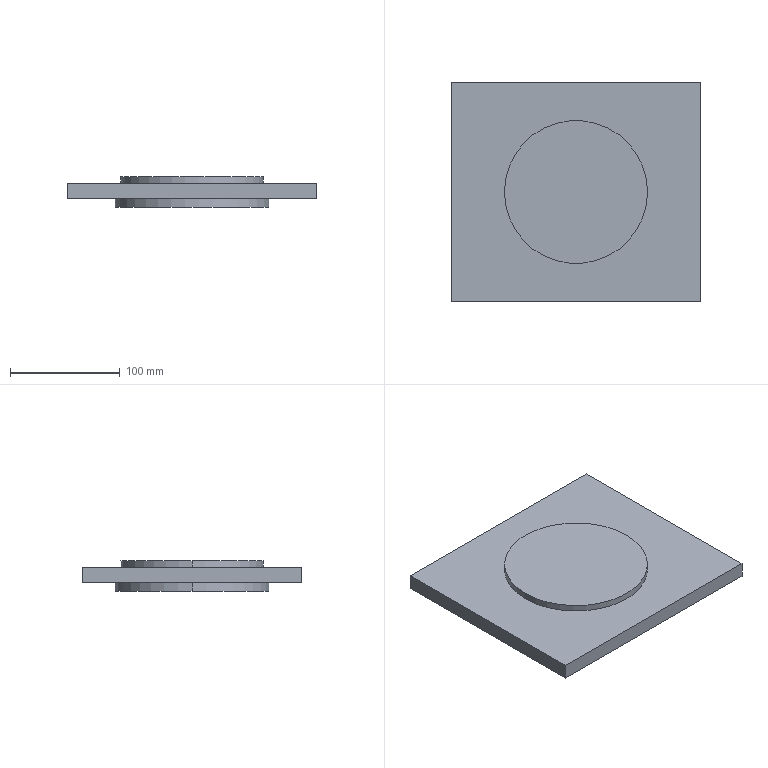Part | SolidWorks | features ICE 2, Extrusion 1 | 1 solid | 12 faces | box 227 x 200 x 28 mm | volume 838390 mm3 | plane 8 | cylinder 4 | commonest cylinder face diameters 130 x2 140 x2
STEP:
#1=CARTESIAN_POINT('',(43.5,100.,-8.));
#2=VERTEX_POINT('',#1);
#3=CARTESIAN_POINT('',(183.5,100.,-8.));
#4=VERTEX_POINT('',#3);
#5=CARTESIAN_POINT('',(113.5,100.,-8.));
#6=DIRECTION('',(0.,0.,-1.));
#7=DIRECTION('',(-1.,0.,0.));
#8=AXIS2_PLACEMENT_3D('',#5,#6,#7);
#9=CIRCLE('',#8,70.);
#10=EDGE_CURVE('',#2,#4,#9,.T.);
#11=ORIENTED_EDGE('',*,*,#10,.F.);
#12=CARTESIAN_POINT('',(43.5,100.,0.));
#13=VERTEX_POINT('',#12);
#14=CARTESIAN_POINT('',(43.5,100.,-8.));
#15=DIRECTION('',(0.,0.,1.));
#16=VECTOR('',#15,1000.);
#17=LINE('',#14,#16);
#18=EDGE_CURVE('',#2,#13,#17,.T.);
#19=ORIENTED_EDGE('',*,*,#18,.T.);
#20=CARTESIAN_POINT('',(183.5,100.,0.));
#21=VERTEX_POINT('',#20);
#22=CARTESIAN_POINT('',(113.5,100.,0.));
#23=DIRECTION('',(0.,0.,-1.));
#24=DIRECTION('',(-1.,0.,0.));
#25=AXIS2_PLACEMENT_3D('',#22,#23,#24);
#26=CIRCLE('',#25,70.);
#27=EDGE_CURVE('',#13,#21,#26,.T.);
#28=ORIENTED_EDGE('',*,*,#27,.T.);
#29=CARTESIAN_POINT('',(183.5,100.,-8.));
#30=DIRECTION('',(0.,0.,1.));
#31=VECTOR('',#30,1000.);
#32=LINE('',#29,#31);
#33=EDGE_CURVE('',#4,#21,#32,.T.);
#34=ORIENTED_EDGE('',*,*,#33,.F.);
#35=EDGE_LOOP('',(#11,#19,#28,#34));
#36=FACE_OUTER_BOUND('',#35,.T.);
#37=CARTESIAN_POINT('',(113.5,100.,-8.));
#38=DIRECTION('',(0.,0.,1.));
#39=DIRECTION('',(1.,0.,0.));
#40=AXIS2_PLACEMENT_3D('',#37,#38,#39);
#41=CYLINDRICAL_SURFACE('',#40,70.);
#42=ADVANCED_FACE('',(#36),#41,.T.);
#43=CARTESIAN_POINT('',(178.5,100.,20.));
#44=VERTEX_POINT('',#43);
#45=CARTESIAN_POINT('',(48.5,100.,20.));
#46=VERTEX_POINT('',#45);
#47=CARTESIAN_POINT('',(113.5,100.,20.));
#48=DIRECTION('',(0.,0.,1.));
#49=DIRECTION('',(1.,0.,0.));
#50=AXIS2_PLACEMENT_3D('',#47,#48,#49);
#51=CIRCLE('',#50,65.);
#52=EDGE_CURVE('',#44,#46,#51,.T.);
#53=ORIENTED_EDGE('',*,*,#52,.F.);
#54=CARTESIAN_POINT('',(178.5,100.,14.));
#55=VERTEX_POINT('',#54);
#56=CARTESIAN_POINT('',(178.5,100.,20.));
#57=DIRECTION('',(0.,0.,-1.));
#58=VECTOR('',#57,1000.);
#59=LINE('',#56,#58);
#60=EDGE_CURVE('',#44,#55,#59,.T.);
#61=ORIENTED_EDGE('',*,*,#60,.T.);
#62=CARTESIAN_POINT('',(48.5,100.,14.));
#63=VERTEX_POINT('',#62);
#64=CARTESIAN_POINT('',(113.5,100.,14.));
#65=DIRECTION('',(0.,0.,1.));
#66=DIRECTION('',(-1.,0.,0.));
#67=AXIS2_PLACEMENT_3D('',#64,#65,#66);
#68=CIRCLE('',#67,65.);
#69=EDGE_CURVE('',#55,#63,#68,.T.);
#70=ORIENTED_EDGE('',*,*,#69,.T.);
#71=CARTESIAN_POINT('',(48.5,100.,20.));
#72=DIRECTION('',(0.,0.,-1.));
#73=VECTOR('',#72,1000.);
#74=LINE('',#71,#73);
#75=EDGE_CURVE('',#46,#63,#74,.T.);
#76=ORIENTED_EDGE('',*,*,#75,.F.);
#77=EDGE_LOOP('',(#53,#61,#70,#76));
#78=FACE_OUTER_BOUND('',#77,.T.);
#79=CARTESIAN_POINT('',(113.5,100.,20.));
#80=DIRECTION('',(0.,0.,-1.));
#81=DIRECTION('',(-1.,0.,0.));
#82=AXIS2_PLACEMENT_3D('',#79,#80,#81);
#83=CYLINDRICAL_SURFACE('',#82,65.);
#84=ADVANCED_FACE('',(#78),#83,.T.);
#85=CARTESIAN_POINT('',(0.,0.,0.));
#86=VERTEX_POINT('',#85);
#87=CARTESIAN_POINT('',(227.,0.,0.));
#88=VERTEX_POINT('',#87);
#89=CARTESIAN_POINT('',(227.,0.,0.));
#90=DIRECTION('',(1.,0.,0.));
#91=VECTOR('',#90,1000.);
#92=LINE('',#89,#91);
#93=EDGE_CURVE('',#86,#88,#92,.T.);
#94=ORIENTED_EDGE('',*,*,#93,.F.);
#95=CARTESIAN_POINT('',(0.,200.,0.));
#96=VERTEX_POINT('',#95);
#97=CARTESIAN_POINT('',(0.,0.,0.));
#98=DIRECTION('',(0.,-1.,0.));
#99=VECTOR('',#98,1000.);
#100=LINE('',#97,#99);
#101=EDGE_CURVE('',#96,#86,#100,.T.);
#102=ORIENTED_EDGE('',*,*,#101,.F.);
#103=CARTESIAN_POINT('',(227.,200.,0.));
#104=VERTEX_POINT('',#103);
#105=CARTESIAN_POINT('',(0.,200.,0.));
#106=DIRECTION('',(-1.,0.,0.));
#107=VECTOR('',#106,1000.);
#108=LINE('',#105,#107);
#109=EDGE_CURVE('',#104,#96,#108,.T.);
#110=ORIENTED_EDGE('',*,*,#109,.F.);
#111=CARTESIAN_POINT('',(227.,200.,0.));
#112=DIRECTION('',(0.,1.,0.));
#113=VECTOR('',#112,1000.);
#114=LINE('',#111,#113);
#115=EDGE_CURVE('',#88,#104,#114,.T.);
#116=ORIENTED_EDGE('',*,*,#115,.F.);
#117=EDGE_LOOP('',(#94,#102,#110,#116));
#118=FACE_OUTER_BOUND('',#117,.T.);
#119=CARTESIAN_POINT('',(113.5,100.,0.));
#120=DIRECTION('',(0.,0.,-1.));
#121=DIRECTION('',(-1.,0.,0.));
#122=AXIS2_PLACEMENT_3D('',#119,#120,#121);
#123=CIRCLE('',#122,70.);
#124=EDGE_CURVE('',#21,#13,#123,.T.);
#125=ORIENTED_EDGE('',*,*,#124,.F.);
#126=ORIENTED_EDGE('',*,*,#27,.F.);
#127=EDGE_LOOP('',(#125,#126));
#128=FACE_BOUND('',#127,.T.);
#129=CARTESIAN_POINT('',(0.,0.,0.));
#130=DIRECTION('',(0.,0.,-1.));
#131=DIRECTION('',(-1.,0.,0.));
#132=AXIS2_PLACEMENT_3D('',#129,#130,#131);
#133=PLANE('',#132);
#134=ADVANCED_FACE('',(#118,#128),#133,.T.);
#135=CARTESIAN_POINT('',(0.,0.,14.));
#136=VERTEX_POINT('',#135);
#137=CARTESIAN_POINT('',(227.,0.,14.));
#138=VERTEX_POINT('',#137);
#139=CARTESIAN_POINT('',(227.,0.,14.));
#140=DIRECTION('',(1.,0.,0.));
#141=VECTOR('',#140,1000.);
#142=LINE('',#139,#141);
#143=EDGE_CURVE('',#136,#138,#142,.T.);
#144=ORIENTED_EDGE('',*,*,#143,.T.);
#145=CARTESIAN_POINT('',(227.,200.,14.));
#146=VERTEX_POINT('',#145);
#147=CARTESIAN_POINT('',(227.,200.,14.));
#148=DIRECTION('',(0.,1.,0.));
#149=VECTOR('',#148,1000.);
#150=LINE('',#147,#149);
#151=EDGE_CURVE('',#138,#146,#150,.T.);
#152=ORIENTED_EDGE('',*,*,#151,.T.);
#153=CARTESIAN_POINT('',(0.,200.,14.));
#154=VERTEX_POINT('',#153);
#155=CARTESIAN_POINT('',(0.,200.,14.));
#156=DIRECTION('',(-1.,0.,0.));
#157=VECTOR('',#156,1000.);
#158=LINE('',#155,#157);
#159=EDGE_CURVE('',#146,#154,#158,.T.);
#160=ORIENTED_EDGE('',*,*,#159,.T.);
#161=CARTESIAN_POINT('',(0.,0.,14.));
#162=DIRECTION('',(0.,-1.,0.));
#163=VECTOR('',#162,1000.);
#164=LINE('',#161,#163);
#165=EDGE_CURVE('',#154,#136,#164,.T.);
#166=ORIENTED_EDGE('',*,*,#165,.T.);
#167=EDGE_LOOP('',(#144,#152,#160,#166));
#168=FACE_OUTER_BOUND('',#167,.T.);
#169=CARTESIAN_POINT('',(113.5,100.,14.));
#170=DIRECTION('',(0.,0.,1.));
#171=DIRECTION('',(-1.,0.,0.));
#172=AXIS2_PLACEMENT_3D('',#169,#170,#171);
#173=CIRCLE('',#172,65.);
#174=EDGE_CURVE('',#63,#55,#173,.T.);
#175=ORIENTED_EDGE('',*,*,#174,.F.);
#176=ORIENTED_EDGE('',*,*,#69,.F.);
#177=EDGE_LOOP('',(#175,#176));
#178=FACE_BOUND('',#177,.T.);
#179=CARTESIAN_POINT('',(0.,0.,14.));
#180=DIRECTION('',(0.,0.,-1.));
#181=DIRECTION('',(-1.,0.,0.));
#182=AXIS2_PLACEMENT_3D('',#179,#180,#181);
#183=PLANE('',#182);
#184=ADVANCED_FACE('',(#168,#178),#183,.F.);
#185=ORIENTED_EDGE('',*,*,#93,.T.);
#186=CARTESIAN_POINT('',(227.,0.,14.));
#187=DIRECTION('',(0.,0.,-1.));
#188=VECTOR('',#187,1000.);
#189=LINE('',#186,#188);
#190=EDGE_CURVE('',#138,#88,#189,.T.);
#191=ORIENTED_EDGE('',*,*,#190,.F.);
#192=ORIENTED_EDGE('',*,*,#143,.F.);
#193=CARTESIAN_POINT('',(0.,0.,14.));
#194=DIRECTION('',(0.,0.,-1.));
#195=VECTOR('',#194,1000.);
#196=LINE('',#193,#195);
#197=EDGE_CURVE('',#136,#86,#196,.T.);
#198=ORIENTED_EDGE('',*,*,#197,.T.);
#199=EDGE_LOOP('',(#185,#191,#192,#198));
#200=FACE_OUTER_BOUND('',#199,.T.);
#201=CARTESIAN_POINT('',(227.,0.,14.));
#202=DIRECTION('',(0.,1.,0.));
#203=DIRECTION('',(-1.,0.,0.));
#204=AXIS2_PLACEMENT_3D('',#201,#202,#203);
#205=PLANE('',#204);
#206=ADVANCED_FACE('',(#200),#205,.F.);
#207=ORIENTED_EDGE('',*,*,#115,.T.);
#208=CARTESIAN_POINT('',(227.,200.,14.));
#209=DIRECTION('',(0.,0.,-1.));
#210=VECTOR('',#209,1000.);
#211=LINE('',#208,#210);
#212=EDGE_CURVE('',#146,#104,#211,.T.);
#213=ORIENTED_EDGE('',*,*,#212,.F.);
#214=ORIENTED_EDGE('',*,*,#151,.F.);
#215=ORIENTED_EDGE('',*,*,#190,.T.);
#216=EDGE_LOOP('',(#207,#213,#214,#215));
#217=FACE_OUTER_BOUND('',#216,.T.);
#218=CARTESIAN_POINT('',(227.,200.,14.));
#219=DIRECTION('',(-1.,0.,0.));
#220=DIRECTION('',(0.,-1.,0.));
#221=AXIS2_PLACEMENT_3D('',#218,#219,#220);
#222=PLANE('',#221);
#223=ADVANCED_FACE('',(#217),#222,.F.);
#224=ORIENTED_EDGE('',*,*,#109,.T.);
#225=CARTESIAN_POINT('',(0.,200.,14.));
#226=DIRECTION('',(0.,0.,-1.));
#227=VECTOR('',#226,1000.);
#228=LINE('',#225,#227);
#229=EDGE_CURVE('',#154,#96,#228,.T.);
#230=ORIENTED_EDGE('',*,*,#229,.F.);
#231=ORIENTED_EDGE('',*,*,#159,.F.);
#232=ORIENTED_EDGE('',*,*,#212,.T.);
#233=EDGE_LOOP('',(#224,#230,#231,#232));
#234=FACE_OUTER_BOUND('',#233,.T.);
#235=CARTESIAN_POINT('',(0.,200.,14.));
#236=DIRECTION('',(0.,-1.,0.));
#237=DIRECTION('',(0.,0.,-1.));
#238=AXIS2_PLACEMENT_3D('',#235,#236,#237);
#239=PLANE('',#238);
#240=ADVANCED_FACE('',(#234),#239,.F.);
#241=ORIENTED_EDGE('',*,*,#101,.T.);
#242=ORIENTED_EDGE('',*,*,#197,.F.);
#243=ORIENTED_EDGE('',*,*,#165,.F.);
#244=ORIENTED_EDGE('',*,*,#229,.T.);
#245=EDGE_LOOP('',(#241,#242,#243,#244));
#246=FACE_OUTER_BOUND('',#245,.T.);
#247=CARTESIAN_POINT('',(0.,0.,14.));
#248=DIRECTION('',(1.,0.,0.));
#249=DIRECTION('',(0.,0.,-1.));
#250=AXIS2_PLACEMENT_3D('',#247,#248,#249);
#251=PLANE('',#250);
#252=ADVANCED_FACE('',(#246),#251,.F.);
#253=ORIENTED_EDGE('',*,*,#60,.F.);
#254=CARTESIAN_POINT('',(113.5,100.,20.));
#255=DIRECTION('',(0.,0.,1.));
#256=DIRECTION('',(1.,0.,0.));
#257=AXIS2_PLACEMENT_3D('',#254,#255,#256);
#258=CIRCLE('',#257,65.);
#259=EDGE_CURVE('',#46,#44,#258,.T.);
#260=ORIENTED_EDGE('',*,*,#259,.F.);
#261=ORIENTED_EDGE('',*,*,#75,.T.);
#262=ORIENTED_EDGE('',*,*,#174,.T.);
#263=EDGE_LOOP('',(#253,#260,#261,#262));
#264=FACE_OUTER_BOUND('',#263,.T.);
#265=CARTESIAN_POINT('',(113.5,100.,20.));
#266=DIRECTION('',(0.,0.,-1.));
#267=DIRECTION('',(-1.,0.,0.));
#268=AXIS2_PLACEMENT_3D('',#265,#266,#267);
#269=CYLINDRICAL_SURFACE('',#268,65.);
#270=ADVANCED_FACE('',(#264),#269,.T.);
#271=ORIENTED_EDGE('',*,*,#259,.T.);
#272=ORIENTED_EDGE('',*,*,#52,.T.);
#273=EDGE_LOOP('',(#271,#272));
#274=FACE_OUTER_BOUND('',#273,.T.);
#275=CARTESIAN_POINT('',(113.5,100.,20.));
#276=DIRECTION('',(0.,0.,1.));
#277=DIRECTION('',(1.,0.,0.));
#278=AXIS2_PLACEMENT_3D('',#275,#276,#277);
#279=PLANE('',#278);
#280=ADVANCED_FACE('',(#274),#279,.T.);
#281=ORIENTED_EDGE('',*,*,#18,.F.);
#282=CARTESIAN_POINT('',(113.5,100.,-8.));
#283=DIRECTION('',(0.,0.,-1.));
#284=DIRECTION('',(-1.,0.,0.));
#285=AXIS2_PLACEMENT_3D('',#282,#283,#284);
#286=CIRCLE('',#285,70.);
#287=EDGE_CURVE('',#4,#2,#286,.T.);
#288=ORIENTED_EDGE('',*,*,#287,.F.);
#289=ORIENTED_EDGE('',*,*,#33,.T.);
#290=ORIENTED_EDGE('',*,*,#124,.T.);
#291=EDGE_LOOP('',(#281,#288,#289,#290));
#292=FACE_OUTER_BOUND('',#291,.T.);
#293=CARTESIAN_POINT('',(113.5,100.,-8.));
#294=DIRECTION('',(0.,0.,1.));
#295=DIRECTION('',(1.,0.,0.));
#296=AXIS2_PLACEMENT_3D('',#293,#294,#295);
#297=CYLINDRICAL_SURFACE('',#296,70.);
#298=ADVANCED_FACE('',(#292),#297,.T.);
#299=ORIENTED_EDGE('',*,*,#287,.T.);
#300=ORIENTED_EDGE('',*,*,#10,.T.);
#301=EDGE_LOOP('',(#299,#300));
#302=FACE_OUTER_BOUND('',#301,.T.);
#303=CARTESIAN_POINT('',(113.5,100.,-8.));
#304=DIRECTION('',(0.,0.,-1.));
#305=DIRECTION('',(-1.,0.,0.));
#306=AXIS2_PLACEMENT_3D('',#303,#304,#305);
#307=PLANE('',#306);
#308=ADVANCED_FACE('',(#302),#307,.T.);
#309=CLOSED_SHELL('',(#42,#84,#134,#184,#206,#223,#240,#252,#270,#280,#298,#308));
#310=MANIFOLD_SOLID_BREP('',#309);
#311=CARTESIAN_POINT('',(0.,0.,0.));
#312=DIRECTION('',(0.,0.,1.));
#313=DIRECTION('',(1.,0.,0.));
#314=AXIS2_PLACEMENT_3D('',#311,#312,#313);
#315=(LENGTH_UNIT()NAMED_UNIT(*)SI_UNIT(.MILLI.,.METRE.));
#316=UNCERTAINTY_MEASURE_WITH_UNIT(LENGTH_MEASURE(0.00001),#315,'','');
#317=(NAMED_UNIT(*)PLANE_ANGLE_UNIT()SI_UNIT($,.RADIAN.));
#318=(NAMED_UNIT(*)SI_UNIT($,.STERADIAN.)SOLID_ANGLE_UNIT());
#319=(GEOMETRIC_REPRESENTATION_CONTEXT(3)GLOBAL_UNCERTAINTY_ASSIGNED_CONTEXT((#316))GLOBAL_UNIT_ASSIGNED_CONTEXT((#315,#317,#318))REPRESENTATION_CONTEXT('',''));
#320=ADVANCED_BREP_SHAPE_REPRESENTATION('',(#310,#314),#319);